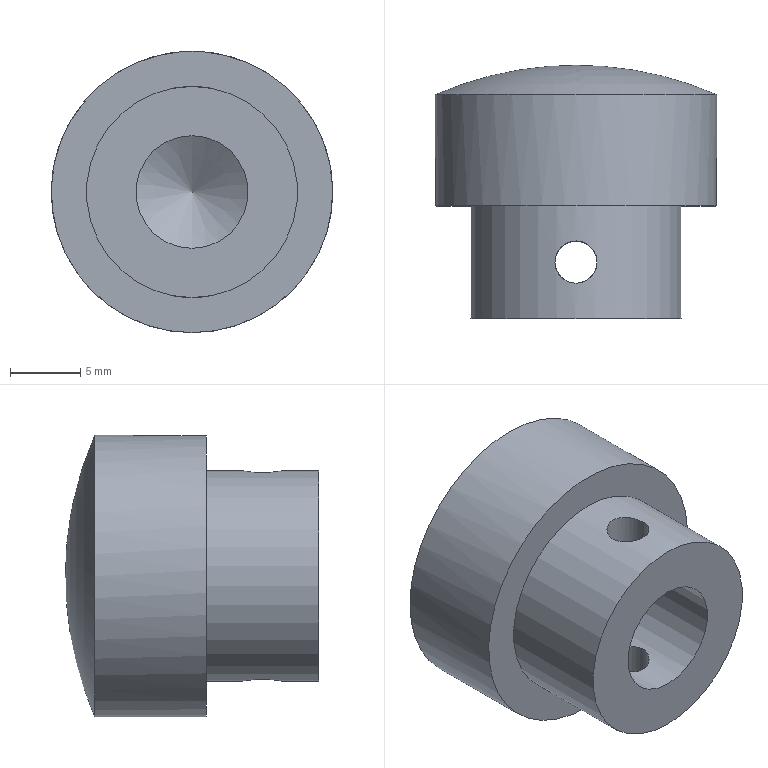Part | NX | features DATUM_CSYS 3, SKETCH 2, EXTRUDE 1, HOLE PACKAGE 1, SIMPLE HOLE 1, SWP104 1 | 1 solid | 9 faces | box 20 x 18 x 20 mm | volume 3740 mm3 | cylinder 5 | plane 2 | sphere 1 | cone 1 | commonest cylinder face diameters 3 x2 8 x1 15 x1 20 x1
STEP:
#1=CARTESIAN_POINT('',(-1.5,4.,3.708));
#2=VERTEX_POINT('',#1);
#3=CARTESIAN_POINT('',(-1.176,5.174,3.859));
#4=CARTESIAN_POINT('',(-1.662,4.,3.632));
#5=CARTESIAN_POINT('',(-1.175,2.825,3.86));
#6=CARTESIAN_POINT('',(-0.002019,2.337,4.07));
#7=CARTESIAN_POINT('',(1.177,2.826,3.859));
#8=CARTESIAN_POINT('',(1.662,3.999,3.632));
#9=CARTESIAN_POINT('',(1.176,5.176,3.86));
#10=CARTESIAN_POINT('',(-0.0004731,5.663,4.07));
#11=CARTESIAN_POINT('',(-1.176,5.174,3.859));
#12=CARTESIAN_POINT('',(-1.662,4.,3.632));
#13=CARTESIAN_POINT('',(-1.175,2.825,3.86));
#14=B_SPLINE_CURVE_WITH_KNOTS('',3,(#3,#4,#5,#6,#7,#8,#9,#10,#11,#12,#13),.UNSPECIFIED.,.T.,.F.,(1,1,1,1,1,1,1,1,1,1,1,1,1,1,1),(-0.003549,-0.002366,-0.001183,0.,0.001183,0.002366,0.003549,0.004733,0.005916,0.007099,0.008282,0.009465,0.01065,0.01183,0.01301),.UNSPECIFIED.);
#15=EDGE_CURVE('',#2,#2,#14,.T.);
#16=ORIENTED_EDGE('',*,*,#15,.F.);
#17=EDGE_LOOP('',(#16));
#18=FACE_BOUND('',#17,.T.);
#19=CARTESIAN_POINT('',(-1.5,4.,7.348));
#20=VERTEX_POINT('',#19);
#21=CARTESIAN_POINT('',(-1.174,5.177,7.425));
#22=CARTESIAN_POINT('',(-1.663,4.,7.31));
#23=CARTESIAN_POINT('',(-1.175,2.824,7.425));
#24=CARTESIAN_POINT('',(-0.001544,2.338,7.537));
#25=CARTESIAN_POINT('',(1.176,2.824,7.425));
#26=CARTESIAN_POINT('',(1.662,3.999,7.31));
#27=CARTESIAN_POINT('',(1.177,5.174,7.425));
#28=CARTESIAN_POINT('',(0.001016,5.662,7.538));
#29=CARTESIAN_POINT('',(-1.174,5.177,7.425));
#30=CARTESIAN_POINT('',(-1.663,4.,7.31));
#31=CARTESIAN_POINT('',(-1.175,2.824,7.425));
#32=B_SPLINE_CURVE_WITH_KNOTS('',3,(#21,#22,#23,#24,#25,#26,#27,#28,#29,#30,#31),.UNSPECIFIED.,.T.,.F.,(1,1,1,1,1,1,1,1,1,1,1,1,1,1,1),(-0.003526,-0.00235,-0.001175,0.,0.001175,0.00235,0.003526,0.004701,0.005876,0.007051,0.008227,0.009402,0.01058,0.01175,0.01293),.UNSPECIFIED.);
#33=EDGE_CURVE('',#20,#20,#32,.T.);
#34=ORIENTED_EDGE('',*,*,#33,.T.);
#35=EDGE_LOOP('',(#34));
#36=FACE_BOUND('',#35,.T.);
#37=CARTESIAN_POINT('',(0.,4.,8.5));
#38=DIRECTION('',(0.,0.,-1.));
#39=DIRECTION('',(-1.,0.,0.));
#40=AXIS2_PLACEMENT_3D('',#37,#38,#39);
#41=CYLINDRICAL_SURFACE('',#40,1.5);
#42=ADVANCED_FACE('',(#18,#36),#41,.F.);
#43=CARTESIAN_POINT('',(0.,0.,-7.5));
#44=VERTEX_POINT('',#43);
#45=CARTESIAN_POINT('',(0.,0.,0.));
#46=DIRECTION('',(0.,-1.,0.));
#47=DIRECTION('',(0.,0.,-1.));
#48=AXIS2_PLACEMENT_3D('',#45,#46,#47);
#49=CIRCLE('',#48,7.5);
#50=EDGE_CURVE('',#44,#44,#49,.T.);
#51=ORIENTED_EDGE('',*,*,#50,.F.);
#52=EDGE_LOOP('',(#51));
#53=FACE_BOUND('',#52,.T.);
#54=CARTESIAN_POINT('',(0.,8.,-7.5));
#55=VERTEX_POINT('',#54);
#56=CARTESIAN_POINT('',(0.,8.,0.));
#57=DIRECTION('',(0.,-1.,0.));
#58=DIRECTION('',(0.,0.,-1.));
#59=AXIS2_PLACEMENT_3D('',#56,#57,#58);
#60=CIRCLE('',#59,7.5);
#61=EDGE_CURVE('',#55,#55,#60,.T.);
#62=ORIENTED_EDGE('',*,*,#61,.T.);
#63=EDGE_LOOP('',(#62));
#64=FACE_BOUND('',#63,.T.);
#65=ORIENTED_EDGE('',*,*,#33,.F.);
#66=EDGE_LOOP('',(#65));
#67=FACE_BOUND('',#66,.T.);
#68=CARTESIAN_POINT('',(0.,5.5,-7.5));
#69=VERTEX_POINT('',#68);
#70=CARTESIAN_POINT('',(-1.177,5.174,-7.425));
#71=CARTESIAN_POINT('',(0.0002626,5.663,-7.538));
#72=CARTESIAN_POINT('',(1.176,5.175,-7.425));
#73=CARTESIAN_POINT('',(1.662,4.002,-7.31));
#74=CARTESIAN_POINT('',(1.176,2.824,-7.425));
#75=CARTESIAN_POINT('',(0.000539,2.338,-7.537));
#76=CARTESIAN_POINT('',(-1.174,2.823,-7.425));
#77=CARTESIAN_POINT('',(-1.662,3.999,-7.31));
#78=CARTESIAN_POINT('',(-1.177,5.174,-7.425));
#79=CARTESIAN_POINT('',(0.0002626,5.663,-7.538));
#80=CARTESIAN_POINT('',(1.176,5.175,-7.425));
#81=B_SPLINE_CURVE_WITH_KNOTS('',3,(#70,#71,#72,#73,#74,#75,#76,#77,#78,#79,#80),.UNSPECIFIED.,.T.,.F.,(1,1,1,1,1,1,1,1,1,1,1,1,1,1,1),(-0.003526,-0.00235,-0.001175,0.,0.001175,0.00235,0.003526,0.004701,0.005876,0.007051,0.008227,0.009402,0.01058,0.01175,0.01293),.UNSPECIFIED.);
#82=EDGE_CURVE('',#69,#69,#81,.T.);
#83=ORIENTED_EDGE('',*,*,#82,.F.);
#84=EDGE_LOOP('',(#83));
#85=FACE_BOUND('',#84,.T.);
#86=CARTESIAN_POINT('',(0.,18.,0.));
#87=DIRECTION('',(0.,-1.,0.));
#88=DIRECTION('',(0.,0.,-1.));
#89=AXIS2_PLACEMENT_3D('',#86,#87,#88);
#90=CYLINDRICAL_SURFACE('',#89,7.5);
#91=ADVANCED_FACE('',(#53,#64,#67,#85),#90,.T.);
#92=CARTESIAN_POINT('',(0.,0.,4.));
#93=VERTEX_POINT('',#92);
#94=CARTESIAN_POINT('',(0.,0.,0.));
#95=DIRECTION('',(0.,1.,0.));
#96=DIRECTION('',(0.,0.,1.));
#97=AXIS2_PLACEMENT_3D('',#94,#95,#96);
#98=CIRCLE('',#97,4.);
#99=EDGE_CURVE('',#93,#93,#98,.T.);
#100=ORIENTED_EDGE('',*,*,#99,.T.);
#101=EDGE_LOOP('',(#100));
#102=FACE_BOUND('',#101,.T.);
#103=ORIENTED_EDGE('',*,*,#50,.T.);
#104=EDGE_LOOP('',(#103));
#105=FACE_BOUND('',#104,.T.);
#106=CARTESIAN_POINT('',(0.,0.,7.5));
#107=DIRECTION('',(0.,1.,0.));
#108=DIRECTION('',(0.,0.,1.));
#109=AXIS2_PLACEMENT_3D('',#106,#107,#108);
#110=PLANE('',#109);
#111=ADVANCED_FACE('',(#102,#105),#110,.F.);
#112=CARTESIAN_POINT('',(0.,15.913,-10.));
#113=VERTEX_POINT('',#112);
#114=CARTESIAN_POINT('',(0.,15.913,0.));
#115=DIRECTION('',(0.,-1.,0.));
#116=DIRECTION('',(0.,0.,-1.));
#117=AXIS2_PLACEMENT_3D('',#114,#115,#116);
#118=CIRCLE('',#117,10.);
#119=EDGE_CURVE('',#113,#113,#118,.T.);
#120=ORIENTED_EDGE('',*,*,#119,.F.);
#121=EDGE_LOOP('',(#120));
#122=FACE_BOUND('',#121,.T.);
#123=CARTESIAN_POINT('',(0.,-7.,0.));
#124=DIRECTION('',(0.,-1.,0.));
#125=DIRECTION('',(0.,0.,1.));
#126=AXIS2_PLACEMENT_3D('',#123,#124,#125);
#127=SPHERICAL_SURFACE('',#126,25.);
#128=ADVANCED_FACE('',(#122),#127,.T.);
#129=CARTESIAN_POINT('',(0.,8.,-10.));
#130=VERTEX_POINT('',#129);
#131=CARTESIAN_POINT('',(0.,8.,0.));
#132=DIRECTION('',(0.,-1.,0.));
#133=DIRECTION('',(0.,0.,-1.));
#134=AXIS2_PLACEMENT_3D('',#131,#132,#133);
#135=CIRCLE('',#134,10.);
#136=EDGE_CURVE('',#130,#130,#135,.T.);
#137=ORIENTED_EDGE('',*,*,#136,.F.);
#138=EDGE_LOOP('',(#137));
#139=FACE_BOUND('',#138,.T.);
#140=ORIENTED_EDGE('',*,*,#119,.T.);
#141=EDGE_LOOP('',(#140));
#142=FACE_BOUND('',#141,.T.);
#143=CARTESIAN_POINT('',(0.,18.,0.));
#144=DIRECTION('',(0.,-1.,0.));
#145=DIRECTION('',(0.,0.,-1.));
#146=AXIS2_PLACEMENT_3D('',#143,#144,#145);
#147=CYLINDRICAL_SURFACE('',#146,10.);
#148=ADVANCED_FACE('',(#139,#142),#147,.T.);
#149=ORIENTED_EDGE('',*,*,#61,.F.);
#150=EDGE_LOOP('',(#149));
#151=FACE_BOUND('',#150,.T.);
#152=ORIENTED_EDGE('',*,*,#136,.T.);
#153=EDGE_LOOP('',(#152));
#154=FACE_BOUND('',#153,.T.);
#155=CARTESIAN_POINT('',(0.,8.,10.));
#156=DIRECTION('',(0.,1.,0.));
#157=DIRECTION('',(0.,0.,1.));
#158=AXIS2_PLACEMENT_3D('',#155,#156,#157);
#159=PLANE('',#158);
#160=ADVANCED_FACE('',(#151,#154),#159,.F.);
#161=CARTESIAN_POINT('',(-1.5,4.,-3.708));
#162=VERTEX_POINT('',#161);
#163=CARTESIAN_POINT('',(-1.176,2.826,-3.859));
#164=CARTESIAN_POINT('',(-1.662,4.,-3.632));
#165=CARTESIAN_POINT('',(-1.175,5.175,-3.86));
#166=CARTESIAN_POINT('',(-0.002019,5.663,-4.07));
#167=CARTESIAN_POINT('',(1.177,5.174,-3.859));
#168=CARTESIAN_POINT('',(1.662,4.001,-3.632));
#169=CARTESIAN_POINT('',(1.176,2.824,-3.86));
#170=CARTESIAN_POINT('',(-0.0004731,2.337,-4.07));
#171=CARTESIAN_POINT('',(-1.176,2.826,-3.859));
#172=CARTESIAN_POINT('',(-1.662,4.,-3.632));
#173=CARTESIAN_POINT('',(-1.175,5.175,-3.86));
#174=B_SPLINE_CURVE_WITH_KNOTS('',3,(#163,#164,#165,#166,#167,#168,#169,#170,#171,#172,#173),.UNSPECIFIED.,.T.,.F.,(1,1,1,1,1,1,1,1,1,1,1,1,1,1,1),(-0.003549,-0.002366,-0.001183,0.,0.001183,0.002366,0.003549,0.004733,0.005916,0.007099,0.008282,0.009465,0.01065,0.01183,0.01301),.UNSPECIFIED.);
#175=EDGE_CURVE('',#162,#162,#174,.T.);
#176=ORIENTED_EDGE('',*,*,#175,.F.);
#177=EDGE_LOOP('',(#176));
#178=FACE_BOUND('',#177,.T.);
#179=ORIENTED_EDGE('',*,*,#82,.T.);
#180=EDGE_LOOP('',(#179));
#181=FACE_BOUND('',#180,.T.);
#182=CARTESIAN_POINT('',(0.,4.,8.5));
#183=DIRECTION('',(0.,0.,-1.));
#184=DIRECTION('',(-1.,0.,0.));
#185=AXIS2_PLACEMENT_3D('',#182,#183,#184);
#186=CYLINDRICAL_SURFACE('',#185,1.5);
#187=ADVANCED_FACE('',(#178,#181),#186,.F.);
#188=CARTESIAN_POINT('',(0.,8.,4.));
#189=VERTEX_POINT('',#188);
#190=CARTESIAN_POINT('',(0.,8.,0.));
#191=DIRECTION('',(0.,1.,0.));
#192=DIRECTION('',(0.,0.,1.));
#193=AXIS2_PLACEMENT_3D('',#190,#191,#192);
#194=CIRCLE('',#193,4.);
#195=EDGE_CURVE('',#189,#189,#194,.F.);
#196=ORIENTED_EDGE('',*,*,#195,.T.);
#197=EDGE_LOOP('',(#196));
#198=FACE_BOUND('',#197,.T.);
#199=CARTESIAN_POINT('',(0.,10.403,0.));
#200=VERTEX_POINT('',#199);
#201=VERTEX_LOOP('',#200);
#202=FACE_BOUND('',#201,.T.);
#203=CARTESIAN_POINT('',(0.,8.,0.));
#204=DIRECTION('',(0.,-1.,0.));
#205=DIRECTION('',(0.,0.,-1.));
#206=AXIS2_PLACEMENT_3D('',#203,#204,#205);
#207=CONICAL_SURFACE('',#206,4.,1.03);
#208=ADVANCED_FACE('',(#198,#202),#207,.F.);
#209=ORIENTED_EDGE('',*,*,#15,.T.);
#210=EDGE_LOOP('',(#209));
#211=FACE_BOUND('',#210,.T.);
#212=ORIENTED_EDGE('',*,*,#175,.T.);
#213=EDGE_LOOP('',(#212));
#214=FACE_BOUND('',#213,.T.);
#215=ORIENTED_EDGE('',*,*,#195,.F.);
#216=EDGE_LOOP('',(#215));
#217=FACE_BOUND('',#216,.T.);
#218=ORIENTED_EDGE('',*,*,#99,.F.);
#219=EDGE_LOOP('',(#218));
#220=FACE_BOUND('',#219,.T.);
#221=CARTESIAN_POINT('',(0.,0.,0.));
#222=DIRECTION('',(0.,1.,0.));
#223=DIRECTION('',(0.,0.,1.));
#224=AXIS2_PLACEMENT_3D('',#221,#222,#223);
#225=CYLINDRICAL_SURFACE('',#224,4.);
#226=ADVANCED_FACE('',(#211,#214,#217,#220),#225,.F.);
#227=CLOSED_SHELL('',(#42,#91,#111,#128,#148,#160,#187,#208,#226));
#228=MANIFOLD_SOLID_BREP('',#227);
#229=(LENGTH_UNIT()NAMED_UNIT(*)SI_UNIT(.MILLI.,.METRE.));
#230=UNCERTAINTY_MEASURE_WITH_UNIT(LENGTH_MEASURE(0.0508),#229,'','');
#231=(NAMED_UNIT(*)PLANE_ANGLE_UNIT()SI_UNIT($,.RADIAN.));
#232=(NAMED_UNIT(*)SI_UNIT($,.STERADIAN.)SOLID_ANGLE_UNIT());
#233=(GEOMETRIC_REPRESENTATION_CONTEXT(3)GLOBAL_UNCERTAINTY_ASSIGNED_CONTEXT((#230))GLOBAL_UNIT_ASSIGNED_CONTEXT((#229,#231,#232))REPRESENTATION_CONTEXT('',''));
#234=ADVANCED_BREP_SHAPE_REPRESENTATION('',(#228),#233);